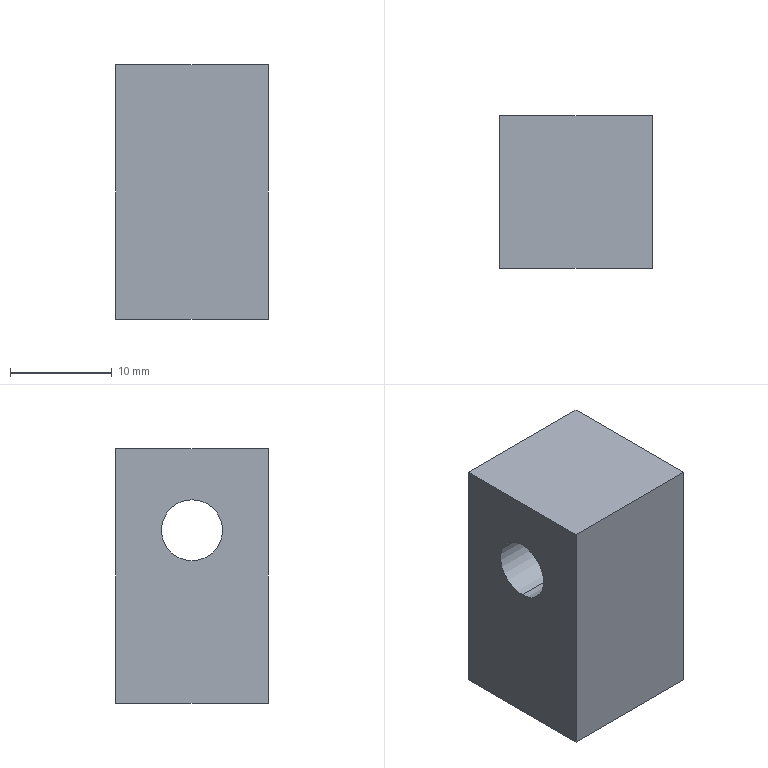Part | SolidWorks | features Cut 1, Extrusion 1 | 1 solid | 8 faces | box 15 x 15 x 25 mm | volume 5201 mm3 | plane 6 | cylinder 2 | commonest cylinder face diameters 6 x2
STEP:
#1=CARTESIAN_POINT('',(7.5,0.,14.));
#2=VERTEX_POINT('',#1);
#3=CARTESIAN_POINT('',(7.5,0.,20.));
#4=VERTEX_POINT('',#3);
#5=CARTESIAN_POINT('',(7.5,0.,17.));
#6=DIRECTION('',(-1.,0.,0.));
#7=DIRECTION('',(0.,0.,1.));
#8=AXIS2_PLACEMENT_3D('',#5,#6,#7);
#9=CIRCLE('',#8,3.);
#10=EDGE_CURVE('',#2,#4,#9,.T.);
#11=ORIENTED_EDGE('',*,*,#10,.F.);
#12=CARTESIAN_POINT('',(-7.5,0.,14.));
#13=VERTEX_POINT('',#12);
#14=CARTESIAN_POINT('',(7.5,0.,14.));
#15=DIRECTION('',(-1.,0.,0.));
#16=VECTOR('',#15,1000.);
#17=LINE('',#14,#16);
#18=EDGE_CURVE('',#2,#13,#17,.T.);
#19=ORIENTED_EDGE('',*,*,#18,.T.);
#20=CARTESIAN_POINT('',(-7.5,0.,20.));
#21=VERTEX_POINT('',#20);
#22=CARTESIAN_POINT('',(-7.5,0.,17.));
#23=DIRECTION('',(1.,0.,0.));
#24=DIRECTION('',(0.,0.,-1.));
#25=AXIS2_PLACEMENT_3D('',#22,#23,#24);
#26=CIRCLE('',#25,3.);
#27=EDGE_CURVE('',#21,#13,#26,.T.);
#28=ORIENTED_EDGE('',*,*,#27,.F.);
#29=CARTESIAN_POINT('',(7.5,0.,20.));
#30=DIRECTION('',(-1.,0.,0.));
#31=VECTOR('',#30,1000.);
#32=LINE('',#29,#31);
#33=EDGE_CURVE('',#4,#21,#32,.T.);
#34=ORIENTED_EDGE('',*,*,#33,.F.);
#35=EDGE_LOOP('',(#11,#19,#28,#34));
#36=FACE_OUTER_BOUND('',#35,.T.);
#37=CARTESIAN_POINT('',(7.5,0.,17.));
#38=DIRECTION('',(-1.,0.,0.));
#39=DIRECTION('',(0.,0.,1.));
#40=AXIS2_PLACEMENT_3D('',#37,#38,#39);
#41=CYLINDRICAL_SURFACE('',#40,3.);
#42=ADVANCED_FACE('',(#36),#41,.F.);
#43=CARTESIAN_POINT('',(7.5,0.,17.));
#44=DIRECTION('',(-1.,0.,0.));
#45=DIRECTION('',(0.,0.,1.));
#46=AXIS2_PLACEMENT_3D('',#43,#44,#45);
#47=CIRCLE('',#46,3.);
#48=EDGE_CURVE('',#4,#2,#47,.T.);
#49=ORIENTED_EDGE('',*,*,#48,.T.);
#50=ORIENTED_EDGE('',*,*,#10,.T.);
#51=EDGE_LOOP('',(#49,#50));
#52=FACE_BOUND('',#51,.T.);
#53=CARTESIAN_POINT('',(7.5,-7.5,0.));
#54=VERTEX_POINT('',#53);
#55=CARTESIAN_POINT('',(7.5,7.5,0.));
#56=VERTEX_POINT('',#55);
#57=CARTESIAN_POINT('',(7.5,7.5,0.));
#58=DIRECTION('',(0.,1.,0.));
#59=VECTOR('',#58,1000.);
#60=LINE('',#57,#59);
#61=EDGE_CURVE('',#54,#56,#60,.T.);
#62=ORIENTED_EDGE('',*,*,#61,.T.);
#63=CARTESIAN_POINT('',(7.5,7.5,25.));
#64=VERTEX_POINT('',#63);
#65=CARTESIAN_POINT('',(7.5,7.5,25.));
#66=DIRECTION('',(0.,0.,-1.));
#67=VECTOR('',#66,1000.);
#68=LINE('',#65,#67);
#69=EDGE_CURVE('',#64,#56,#68,.T.);
#70=ORIENTED_EDGE('',*,*,#69,.F.);
#71=CARTESIAN_POINT('',(7.5,-7.5,25.));
#72=VERTEX_POINT('',#71);
#73=CARTESIAN_POINT('',(7.5,7.5,25.));
#74=DIRECTION('',(0.,1.,0.));
#75=VECTOR('',#74,1000.);
#76=LINE('',#73,#75);
#77=EDGE_CURVE('',#72,#64,#76,.T.);
#78=ORIENTED_EDGE('',*,*,#77,.F.);
#79=CARTESIAN_POINT('',(7.5,-7.5,25.));
#80=DIRECTION('',(0.,0.,-1.));
#81=VECTOR('',#80,1000.);
#82=LINE('',#79,#81);
#83=EDGE_CURVE('',#72,#54,#82,.T.);
#84=ORIENTED_EDGE('',*,*,#83,.T.);
#85=EDGE_LOOP('',(#62,#70,#78,#84));
#86=FACE_OUTER_BOUND('',#85,.T.);
#87=CARTESIAN_POINT('',(7.5,7.5,25.));
#88=DIRECTION('',(-1.,0.,0.));
#89=DIRECTION('',(0.,0.,1.));
#90=AXIS2_PLACEMENT_3D('',#87,#88,#89);
#91=PLANE('',#90);
#92=ADVANCED_FACE('',(#52,#86),#91,.F.);
#93=CARTESIAN_POINT('',(-7.5,7.5,0.));
#94=VERTEX_POINT('',#93);
#95=CARTESIAN_POINT('',(-7.5,7.5,0.));
#96=DIRECTION('',(-1.,0.,0.));
#97=VECTOR('',#96,1000.);
#98=LINE('',#95,#97);
#99=EDGE_CURVE('',#56,#94,#98,.T.);
#100=ORIENTED_EDGE('',*,*,#99,.T.);
#101=CARTESIAN_POINT('',(-7.5,7.5,25.));
#102=VERTEX_POINT('',#101);
#103=CARTESIAN_POINT('',(-7.5,7.5,25.));
#104=DIRECTION('',(0.,0.,-1.));
#105=VECTOR('',#104,1000.);
#106=LINE('',#103,#105);
#107=EDGE_CURVE('',#102,#94,#106,.T.);
#108=ORIENTED_EDGE('',*,*,#107,.F.);
#109=CARTESIAN_POINT('',(-7.5,7.5,25.));
#110=DIRECTION('',(-1.,0.,0.));
#111=VECTOR('',#110,1000.);
#112=LINE('',#109,#111);
#113=EDGE_CURVE('',#64,#102,#112,.T.);
#114=ORIENTED_EDGE('',*,*,#113,.F.);
#115=ORIENTED_EDGE('',*,*,#69,.T.);
#116=EDGE_LOOP('',(#100,#108,#114,#115));
#117=FACE_OUTER_BOUND('',#116,.T.);
#118=CARTESIAN_POINT('',(-7.5,7.5,25.));
#119=DIRECTION('',(0.,-1.,0.));
#120=DIRECTION('',(0.,0.,-1.));
#121=AXIS2_PLACEMENT_3D('',#118,#119,#120);
#122=PLANE('',#121);
#123=ADVANCED_FACE('',(#117),#122,.F.);
#124=ORIENTED_EDGE('',*,*,#27,.T.);
#125=CARTESIAN_POINT('',(-7.5,0.,17.));
#126=DIRECTION('',(1.,0.,0.));
#127=DIRECTION('',(0.,0.,-1.));
#128=AXIS2_PLACEMENT_3D('',#125,#126,#127);
#129=CIRCLE('',#128,3.);
#130=EDGE_CURVE('',#13,#21,#129,.T.);
#131=ORIENTED_EDGE('',*,*,#130,.T.);
#132=EDGE_LOOP('',(#124,#131));
#133=FACE_BOUND('',#132,.T.);
#134=CARTESIAN_POINT('',(-7.5,-7.5,0.));
#135=VERTEX_POINT('',#134);
#136=CARTESIAN_POINT('',(-7.5,7.5,0.));
#137=DIRECTION('',(0.,-1.,0.));
#138=VECTOR('',#137,1000.);
#139=LINE('',#136,#138);
#140=EDGE_CURVE('',#94,#135,#139,.T.);
#141=ORIENTED_EDGE('',*,*,#140,.T.);
#142=CARTESIAN_POINT('',(-7.5,-7.5,25.));
#143=VERTEX_POINT('',#142);
#144=CARTESIAN_POINT('',(-7.5,-7.5,25.));
#145=DIRECTION('',(0.,0.,-1.));
#146=VECTOR('',#145,1000.);
#147=LINE('',#144,#146);
#148=EDGE_CURVE('',#143,#135,#147,.T.);
#149=ORIENTED_EDGE('',*,*,#148,.F.);
#150=CARTESIAN_POINT('',(-7.5,7.5,25.));
#151=DIRECTION('',(0.,-1.,0.));
#152=VECTOR('',#151,1000.);
#153=LINE('',#150,#152);
#154=EDGE_CURVE('',#102,#143,#153,.T.);
#155=ORIENTED_EDGE('',*,*,#154,.F.);
#156=ORIENTED_EDGE('',*,*,#107,.T.);
#157=EDGE_LOOP('',(#141,#149,#155,#156));
#158=FACE_OUTER_BOUND('',#157,.T.);
#159=CARTESIAN_POINT('',(-7.5,7.5,25.));
#160=DIRECTION('',(1.,0.,0.));
#161=DIRECTION('',(0.,0.,-1.));
#162=AXIS2_PLACEMENT_3D('',#159,#160,#161);
#163=PLANE('',#162);
#164=ADVANCED_FACE('',(#133,#158),#163,.F.);
#165=CARTESIAN_POINT('',(-7.5,-7.5,0.));
#166=DIRECTION('',(1.,0.,0.));
#167=VECTOR('',#166,1000.);
#168=LINE('',#165,#167);
#169=EDGE_CURVE('',#135,#54,#168,.T.);
#170=ORIENTED_EDGE('',*,*,#169,.T.);
#171=ORIENTED_EDGE('',*,*,#83,.F.);
#172=CARTESIAN_POINT('',(-7.5,-7.5,25.));
#173=DIRECTION('',(1.,0.,0.));
#174=VECTOR('',#173,1000.);
#175=LINE('',#172,#174);
#176=EDGE_CURVE('',#143,#72,#175,.T.);
#177=ORIENTED_EDGE('',*,*,#176,.F.);
#178=ORIENTED_EDGE('',*,*,#148,.T.);
#179=EDGE_LOOP('',(#170,#171,#177,#178));
#180=FACE_OUTER_BOUND('',#179,.T.);
#181=CARTESIAN_POINT('',(-7.5,-7.5,25.));
#182=DIRECTION('',(0.,1.,0.));
#183=DIRECTION('',(0.,0.,1.));
#184=AXIS2_PLACEMENT_3D('',#181,#182,#183);
#185=PLANE('',#184);
#186=ADVANCED_FACE('',(#180),#185,.F.);
#187=ORIENTED_EDGE('',*,*,#77,.T.);
#188=ORIENTED_EDGE('',*,*,#113,.T.);
#189=ORIENTED_EDGE('',*,*,#154,.T.);
#190=ORIENTED_EDGE('',*,*,#176,.T.);
#191=EDGE_LOOP('',(#187,#188,#189,#190));
#192=FACE_OUTER_BOUND('',#191,.T.);
#193=CARTESIAN_POINT('',(0.,0.,25.));
#194=DIRECTION('',(0.,0.,1.));
#195=DIRECTION('',(1.,0.,0.));
#196=AXIS2_PLACEMENT_3D('',#193,#194,#195);
#197=PLANE('',#196);
#198=ADVANCED_FACE('',(#192),#197,.T.);
#199=ORIENTED_EDGE('',*,*,#61,.F.);
#200=ORIENTED_EDGE('',*,*,#169,.F.);
#201=ORIENTED_EDGE('',*,*,#140,.F.);
#202=ORIENTED_EDGE('',*,*,#99,.F.);
#203=EDGE_LOOP('',(#199,#200,#201,#202));
#204=FACE_OUTER_BOUND('',#203,.T.);
#205=CARTESIAN_POINT('',(0.,0.,0.));
#206=DIRECTION('',(0.,0.,1.));
#207=DIRECTION('',(1.,0.,0.));
#208=AXIS2_PLACEMENT_3D('',#205,#206,#207);
#209=PLANE('',#208);
#210=ADVANCED_FACE('',(#204),#209,.F.);
#211=ORIENTED_EDGE('',*,*,#18,.F.);
#212=ORIENTED_EDGE('',*,*,#48,.F.);
#213=ORIENTED_EDGE('',*,*,#33,.T.);
#214=ORIENTED_EDGE('',*,*,#130,.F.);
#215=EDGE_LOOP('',(#211,#212,#213,#214));
#216=FACE_OUTER_BOUND('',#215,.T.);
#217=CARTESIAN_POINT('',(7.5,0.,17.));
#218=DIRECTION('',(-1.,0.,0.));
#219=DIRECTION('',(0.,0.,1.));
#220=AXIS2_PLACEMENT_3D('',#217,#218,#219);
#221=CYLINDRICAL_SURFACE('',#220,3.);
#222=ADVANCED_FACE('',(#216),#221,.F.);
#223=CLOSED_SHELL('',(#42,#92,#123,#164,#186,#198,#210,#222));
#224=MANIFOLD_SOLID_BREP('',#223);
#225=CARTESIAN_POINT('',(0.,0.,0.));
#226=DIRECTION('',(0.,0.,1.));
#227=DIRECTION('',(1.,0.,0.));
#228=AXIS2_PLACEMENT_3D('',#225,#226,#227);
#229=(LENGTH_UNIT()NAMED_UNIT(*)SI_UNIT(.MILLI.,.METRE.));
#230=UNCERTAINTY_MEASURE_WITH_UNIT(LENGTH_MEASURE(0.00001),#229,'','');
#231=(NAMED_UNIT(*)PLANE_ANGLE_UNIT()SI_UNIT($,.RADIAN.));
#232=(NAMED_UNIT(*)SI_UNIT($,.STERADIAN.)SOLID_ANGLE_UNIT());
#233=(GEOMETRIC_REPRESENTATION_CONTEXT(3)GLOBAL_UNCERTAINTY_ASSIGNED_CONTEXT((#230))GLOBAL_UNIT_ASSIGNED_CONTEXT((#229,#231,#232))REPRESENTATION_CONTEXT('',''));
#234=ADVANCED_BREP_SHAPE_REPRESENTATION('',(#224,#228),#233);